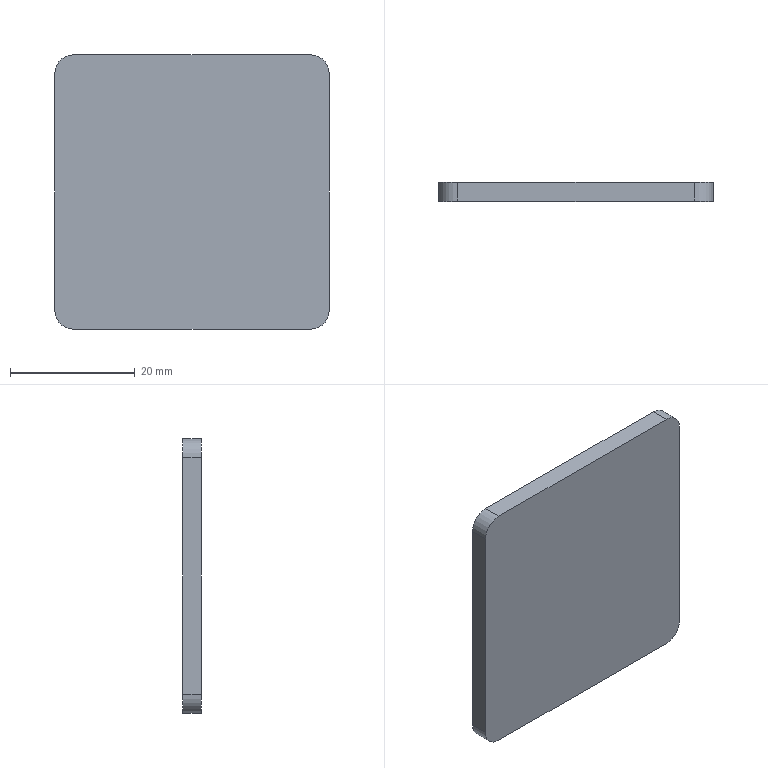Part | SolidWorks | features Extrusion 1, Fillet 1 | 1 solid | 10 faces | box 44 x 3 x 44 mm | volume 5785 mm3 | plane 6 | cylinder 4 | commonest cylinder face diameters 6 x4
STEP:
#1=CARTESIAN_POINT('',(22.,0.,19.));
#2=VERTEX_POINT('',#1);
#3=CARTESIAN_POINT('',(22.,0.,-19.));
#4=VERTEX_POINT('',#3);
#5=CARTESIAN_POINT('',(22.,0.,-22.));
#6=DIRECTION('',(0.,0.,-1.));
#7=VECTOR('',#6,1000.);
#8=LINE('',#5,#7);
#9=EDGE_CURVE('',#2,#4,#8,.T.);
#10=ORIENTED_EDGE('',*,*,#9,.T.);
#11=CARTESIAN_POINT('',(22.,3.,-19.));
#12=VERTEX_POINT('',#11);
#13=CARTESIAN_POINT('',(22.,3.,-19.));
#14=DIRECTION('',(0.,1.,0.));
#15=VECTOR('',#14,1000.);
#16=LINE('',#13,#15);
#17=EDGE_CURVE('',#4,#12,#16,.T.);
#18=ORIENTED_EDGE('',*,*,#17,.T.);
#19=CARTESIAN_POINT('',(22.,3.,19.));
#20=VERTEX_POINT('',#19);
#21=CARTESIAN_POINT('',(22.,3.,-22.));
#22=DIRECTION('',(0.,0.,-1.));
#23=VECTOR('',#22,1000.);
#24=LINE('',#21,#23);
#25=EDGE_CURVE('',#20,#12,#24,.T.);
#26=ORIENTED_EDGE('',*,*,#25,.F.);
#27=CARTESIAN_POINT('',(22.,3.,19.));
#28=DIRECTION('',(0.,-1.,0.));
#29=VECTOR('',#28,1000.);
#30=LINE('',#27,#29);
#31=EDGE_CURVE('',#20,#2,#30,.T.);
#32=ORIENTED_EDGE('',*,*,#31,.T.);
#33=EDGE_LOOP('',(#10,#18,#26,#32));
#34=FACE_OUTER_BOUND('',#33,.T.);
#35=CARTESIAN_POINT('',(22.,3.,-22.));
#36=DIRECTION('',(-1.,0.,0.));
#37=DIRECTION('',(0.,0.,1.));
#38=AXIS2_PLACEMENT_3D('',#35,#36,#37);
#39=PLANE('',#38);
#40=ADVANCED_FACE('',(#34),#39,.F.);
#41=CARTESIAN_POINT('',(19.,0.,-22.));
#42=VERTEX_POINT('',#41);
#43=CARTESIAN_POINT('',(-19.,0.,-22.));
#44=VERTEX_POINT('',#43);
#45=CARTESIAN_POINT('',(-22.,0.,-22.));
#46=DIRECTION('',(-1.,0.,0.));
#47=VECTOR('',#46,1000.);
#48=LINE('',#45,#47);
#49=EDGE_CURVE('',#42,#44,#48,.T.);
#50=ORIENTED_EDGE('',*,*,#49,.T.);
#51=CARTESIAN_POINT('',(-19.,3.,-22.));
#52=VERTEX_POINT('',#51);
#53=CARTESIAN_POINT('',(-19.,3.,-22.));
#54=DIRECTION('',(0.,1.,0.));
#55=VECTOR('',#54,1000.);
#56=LINE('',#53,#55);
#57=EDGE_CURVE('',#44,#52,#56,.T.);
#58=ORIENTED_EDGE('',*,*,#57,.T.);
#59=CARTESIAN_POINT('',(19.,3.,-22.));
#60=VERTEX_POINT('',#59);
#61=CARTESIAN_POINT('',(-22.,3.,-22.));
#62=DIRECTION('',(-1.,0.,0.));
#63=VECTOR('',#62,1000.);
#64=LINE('',#61,#63);
#65=EDGE_CURVE('',#60,#52,#64,.T.);
#66=ORIENTED_EDGE('',*,*,#65,.F.);
#67=CARTESIAN_POINT('',(19.,3.,-22.));
#68=DIRECTION('',(0.,-1.,0.));
#69=VECTOR('',#68,1000.);
#70=LINE('',#67,#69);
#71=EDGE_CURVE('',#60,#42,#70,.T.);
#72=ORIENTED_EDGE('',*,*,#71,.T.);
#73=EDGE_LOOP('',(#50,#58,#66,#72));
#74=FACE_OUTER_BOUND('',#73,.T.);
#75=CARTESIAN_POINT('',(-22.,3.,-22.));
#76=DIRECTION('',(0.,0.,1.));
#77=DIRECTION('',(1.,0.,0.));
#78=AXIS2_PLACEMENT_3D('',#75,#76,#77);
#79=PLANE('',#78);
#80=ADVANCED_FACE('',(#74),#79,.F.);
#81=CARTESIAN_POINT('',(-22.,3.,-19.));
#82=VERTEX_POINT('',#81);
#83=CARTESIAN_POINT('',(-22.,3.,19.));
#84=VERTEX_POINT('',#83);
#85=CARTESIAN_POINT('',(-22.,3.,-22.));
#86=DIRECTION('',(0.,0.,1.));
#87=VECTOR('',#86,1000.);
#88=LINE('',#85,#87);
#89=EDGE_CURVE('',#82,#84,#88,.T.);
#90=ORIENTED_EDGE('',*,*,#89,.F.);
#91=CARTESIAN_POINT('',(-22.,0.,-19.));
#92=VERTEX_POINT('',#91);
#93=CARTESIAN_POINT('',(-22.,3.,-19.));
#94=DIRECTION('',(0.,-1.,0.));
#95=VECTOR('',#94,1000.);
#96=LINE('',#93,#95);
#97=EDGE_CURVE('',#82,#92,#96,.T.);
#98=ORIENTED_EDGE('',*,*,#97,.T.);
#99=CARTESIAN_POINT('',(-22.,0.,19.));
#100=VERTEX_POINT('',#99);
#101=CARTESIAN_POINT('',(-22.,0.,-22.));
#102=DIRECTION('',(0.,0.,1.));
#103=VECTOR('',#102,1000.);
#104=LINE('',#101,#103);
#105=EDGE_CURVE('',#92,#100,#104,.T.);
#106=ORIENTED_EDGE('',*,*,#105,.T.);
#107=CARTESIAN_POINT('',(-22.,3.,19.));
#108=DIRECTION('',(0.,1.,0.));
#109=VECTOR('',#108,1000.);
#110=LINE('',#107,#109);
#111=EDGE_CURVE('',#100,#84,#110,.T.);
#112=ORIENTED_EDGE('',*,*,#111,.T.);
#113=EDGE_LOOP('',(#90,#98,#106,#112));
#114=FACE_OUTER_BOUND('',#113,.T.);
#115=CARTESIAN_POINT('',(-22.,3.,-22.));
#116=DIRECTION('',(1.,0.,0.));
#117=DIRECTION('',(0.,0.,-1.));
#118=AXIS2_PLACEMENT_3D('',#115,#116,#117);
#119=PLANE('',#118);
#120=ADVANCED_FACE('',(#114),#119,.F.);
#121=CARTESIAN_POINT('',(-19.,0.,22.));
#122=VERTEX_POINT('',#121);
#123=CARTESIAN_POINT('',(19.,0.,22.));
#124=VERTEX_POINT('',#123);
#125=CARTESIAN_POINT('',(-22.,0.,22.));
#126=DIRECTION('',(1.,0.,0.));
#127=VECTOR('',#126,1000.);
#128=LINE('',#125,#127);
#129=EDGE_CURVE('',#122,#124,#128,.T.);
#130=ORIENTED_EDGE('',*,*,#129,.T.);
#131=CARTESIAN_POINT('',(19.,3.,22.));
#132=VERTEX_POINT('',#131);
#133=CARTESIAN_POINT('',(19.,3.,22.));
#134=DIRECTION('',(0.,1.,0.));
#135=VECTOR('',#134,1000.);
#136=LINE('',#133,#135);
#137=EDGE_CURVE('',#124,#132,#136,.T.);
#138=ORIENTED_EDGE('',*,*,#137,.T.);
#139=CARTESIAN_POINT('',(-19.,3.,22.));
#140=VERTEX_POINT('',#139);
#141=CARTESIAN_POINT('',(-22.,3.,22.));
#142=DIRECTION('',(1.,0.,0.));
#143=VECTOR('',#142,1000.);
#144=LINE('',#141,#143);
#145=EDGE_CURVE('',#140,#132,#144,.T.);
#146=ORIENTED_EDGE('',*,*,#145,.F.);
#147=CARTESIAN_POINT('',(-19.,3.,22.));
#148=DIRECTION('',(0.,-1.,0.));
#149=VECTOR('',#148,1000.);
#150=LINE('',#147,#149);
#151=EDGE_CURVE('',#140,#122,#150,.T.);
#152=ORIENTED_EDGE('',*,*,#151,.T.);
#153=EDGE_LOOP('',(#130,#138,#146,#152));
#154=FACE_OUTER_BOUND('',#153,.T.);
#155=CARTESIAN_POINT('',(-22.,3.,22.));
#156=DIRECTION('',(0.,0.,-1.));
#157=DIRECTION('',(-1.,0.,0.));
#158=AXIS2_PLACEMENT_3D('',#155,#156,#157);
#159=PLANE('',#158);
#160=ADVANCED_FACE('',(#154),#159,.F.);
#161=ORIENTED_EDGE('',*,*,#65,.T.);
#162=CARTESIAN_POINT('',(-19.,3.,-19.));
#163=DIRECTION('',(0.,1.,0.));
#164=DIRECTION('',(0.,0.,1.));
#165=AXIS2_PLACEMENT_3D('',#162,#163,#164);
#166=CIRCLE('',#165,3.);
#167=EDGE_CURVE('',#52,#82,#166,.T.);
#168=ORIENTED_EDGE('',*,*,#167,.T.);
#169=ORIENTED_EDGE('',*,*,#89,.T.);
#170=CARTESIAN_POINT('',(-19.,3.,19.));
#171=DIRECTION('',(0.,1.,0.));
#172=DIRECTION('',(0.,0.,1.));
#173=AXIS2_PLACEMENT_3D('',#170,#171,#172);
#174=CIRCLE('',#173,3.);
#175=EDGE_CURVE('',#84,#140,#174,.T.);
#176=ORIENTED_EDGE('',*,*,#175,.T.);
#177=ORIENTED_EDGE('',*,*,#145,.T.);
#178=CARTESIAN_POINT('',(19.,3.,19.));
#179=DIRECTION('',(0.,1.,0.));
#180=DIRECTION('',(0.,0.,1.));
#181=AXIS2_PLACEMENT_3D('',#178,#179,#180);
#182=CIRCLE('',#181,3.);
#183=EDGE_CURVE('',#132,#20,#182,.T.);
#184=ORIENTED_EDGE('',*,*,#183,.T.);
#185=ORIENTED_EDGE('',*,*,#25,.T.);
#186=CARTESIAN_POINT('',(19.,3.,-19.));
#187=DIRECTION('',(0.,1.,0.));
#188=DIRECTION('',(0.,0.,1.));
#189=AXIS2_PLACEMENT_3D('',#186,#187,#188);
#190=CIRCLE('',#189,3.);
#191=EDGE_CURVE('',#12,#60,#190,.T.);
#192=ORIENTED_EDGE('',*,*,#191,.T.);
#193=EDGE_LOOP('',(#161,#168,#169,#176,#177,#184,#185,#192));
#194=FACE_OUTER_BOUND('',#193,.T.);
#195=CARTESIAN_POINT('',(0.,3.,0.));
#196=DIRECTION('',(0.,1.,0.));
#197=DIRECTION('',(0.,0.,1.));
#198=AXIS2_PLACEMENT_3D('',#195,#196,#197);
#199=PLANE('',#198);
#200=ADVANCED_FACE('',(#194),#199,.T.);
#201=ORIENTED_EDGE('',*,*,#105,.F.);
#202=CARTESIAN_POINT('',(-19.,0.,-19.));
#203=DIRECTION('',(0.,-1.,0.));
#204=DIRECTION('',(0.,0.,1.));
#205=AXIS2_PLACEMENT_3D('',#202,#203,#204);
#206=CIRCLE('',#205,3.);
#207=EDGE_CURVE('',#92,#44,#206,.T.);
#208=ORIENTED_EDGE('',*,*,#207,.T.);
#209=ORIENTED_EDGE('',*,*,#49,.F.);
#210=CARTESIAN_POINT('',(19.,0.,-19.));
#211=DIRECTION('',(0.,-1.,0.));
#212=DIRECTION('',(0.,0.,1.));
#213=AXIS2_PLACEMENT_3D('',#210,#211,#212);
#214=CIRCLE('',#213,3.);
#215=EDGE_CURVE('',#42,#4,#214,.T.);
#216=ORIENTED_EDGE('',*,*,#215,.T.);
#217=ORIENTED_EDGE('',*,*,#9,.F.);
#218=CARTESIAN_POINT('',(19.,0.,19.));
#219=DIRECTION('',(0.,-1.,0.));
#220=DIRECTION('',(0.,0.,1.));
#221=AXIS2_PLACEMENT_3D('',#218,#219,#220);
#222=CIRCLE('',#221,3.);
#223=EDGE_CURVE('',#2,#124,#222,.T.);
#224=ORIENTED_EDGE('',*,*,#223,.T.);
#225=ORIENTED_EDGE('',*,*,#129,.F.);
#226=CARTESIAN_POINT('',(-19.,0.,19.));
#227=DIRECTION('',(0.,-1.,0.));
#228=DIRECTION('',(0.,0.,1.));
#229=AXIS2_PLACEMENT_3D('',#226,#227,#228);
#230=CIRCLE('',#229,3.);
#231=EDGE_CURVE('',#122,#100,#230,.T.);
#232=ORIENTED_EDGE('',*,*,#231,.T.);
#233=EDGE_LOOP('',(#201,#208,#209,#216,#217,#224,#225,#232));
#234=FACE_OUTER_BOUND('',#233,.T.);
#235=CARTESIAN_POINT('',(0.,0.,0.));
#236=DIRECTION('',(0.,1.,0.));
#237=DIRECTION('',(0.,0.,1.));
#238=AXIS2_PLACEMENT_3D('',#235,#236,#237);
#239=PLANE('',#238);
#240=ADVANCED_FACE('',(#234),#239,.F.);
#241=ORIENTED_EDGE('',*,*,#167,.F.);
#242=ORIENTED_EDGE('',*,*,#57,.F.);
#243=ORIENTED_EDGE('',*,*,#207,.F.);
#244=ORIENTED_EDGE('',*,*,#97,.F.);
#245=EDGE_LOOP('',(#241,#242,#243,#244));
#246=FACE_OUTER_BOUND('',#245,.T.);
#247=CARTESIAN_POINT('',(-19.,3.,-19.));
#248=DIRECTION('',(0.,-1.,0.));
#249=DIRECTION('',(0.,0.,-1.));
#250=AXIS2_PLACEMENT_3D('',#247,#248,#249);
#251=CYLINDRICAL_SURFACE('',#250,3.);
#252=ADVANCED_FACE('',(#246),#251,.T.);
#253=ORIENTED_EDGE('',*,*,#191,.F.);
#254=ORIENTED_EDGE('',*,*,#17,.F.);
#255=ORIENTED_EDGE('',*,*,#215,.F.);
#256=ORIENTED_EDGE('',*,*,#71,.F.);
#257=EDGE_LOOP('',(#253,#254,#255,#256));
#258=FACE_OUTER_BOUND('',#257,.T.);
#259=CARTESIAN_POINT('',(19.,3.,-19.));
#260=DIRECTION('',(0.,-1.,0.));
#261=DIRECTION('',(0.,0.,-1.));
#262=AXIS2_PLACEMENT_3D('',#259,#260,#261);
#263=CYLINDRICAL_SURFACE('',#262,3.);
#264=ADVANCED_FACE('',(#258),#263,.T.);
#265=ORIENTED_EDGE('',*,*,#183,.F.);
#266=ORIENTED_EDGE('',*,*,#137,.F.);
#267=ORIENTED_EDGE('',*,*,#223,.F.);
#268=ORIENTED_EDGE('',*,*,#31,.F.);
#269=EDGE_LOOP('',(#265,#266,#267,#268));
#270=FACE_OUTER_BOUND('',#269,.T.);
#271=CARTESIAN_POINT('',(19.,3.,19.));
#272=DIRECTION('',(0.,-1.,0.));
#273=DIRECTION('',(0.,0.,-1.));
#274=AXIS2_PLACEMENT_3D('',#271,#272,#273);
#275=CYLINDRICAL_SURFACE('',#274,3.);
#276=ADVANCED_FACE('',(#270),#275,.T.);
#277=ORIENTED_EDGE('',*,*,#175,.F.);
#278=ORIENTED_EDGE('',*,*,#111,.F.);
#279=ORIENTED_EDGE('',*,*,#231,.F.);
#280=ORIENTED_EDGE('',*,*,#151,.F.);
#281=EDGE_LOOP('',(#277,#278,#279,#280));
#282=FACE_OUTER_BOUND('',#281,.T.);
#283=CARTESIAN_POINT('',(-19.,3.,19.));
#284=DIRECTION('',(0.,-1.,0.));
#285=DIRECTION('',(0.,0.,-1.));
#286=AXIS2_PLACEMENT_3D('',#283,#284,#285);
#287=CYLINDRICAL_SURFACE('',#286,3.);
#288=ADVANCED_FACE('',(#282),#287,.T.);
#289=CLOSED_SHELL('',(#40,#80,#120,#160,#200,#240,#252,#264,#276,#288));
#290=MANIFOLD_SOLID_BREP('',#289);
#291=CARTESIAN_POINT('',(0.,0.,0.));
#292=DIRECTION('',(0.,0.,1.));
#293=DIRECTION('',(1.,0.,0.));
#294=AXIS2_PLACEMENT_3D('',#291,#292,#293);
#295=(LENGTH_UNIT()NAMED_UNIT(*)SI_UNIT(.MILLI.,.METRE.));
#296=UNCERTAINTY_MEASURE_WITH_UNIT(LENGTH_MEASURE(0.00001),#295,'','');
#297=(NAMED_UNIT(*)PLANE_ANGLE_UNIT()SI_UNIT($,.RADIAN.));
#298=(NAMED_UNIT(*)SI_UNIT($,.STERADIAN.)SOLID_ANGLE_UNIT());
#299=(GEOMETRIC_REPRESENTATION_CONTEXT(3)GLOBAL_UNCERTAINTY_ASSIGNED_CONTEXT((#296))GLOBAL_UNIT_ASSIGNED_CONTEXT((#295,#297,#298))REPRESENTATION_CONTEXT('',''));
#300=ADVANCED_BREP_SHAPE_REPRESENTATION('',(#290,#294),#299);